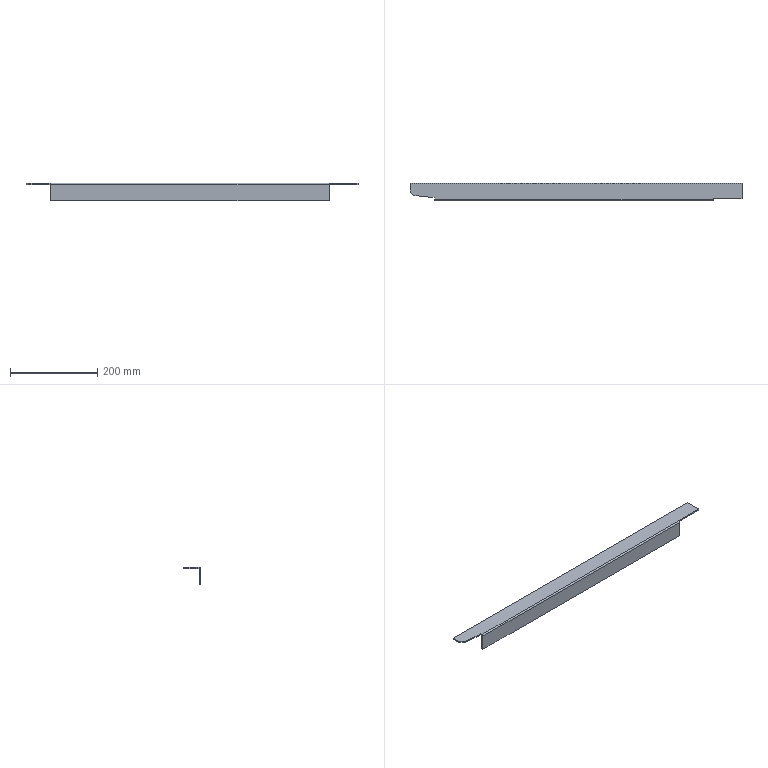Part | SolidWorks | 1 solid | 20 faces | box 759.5 x 40 x 40 mm | volume 157924 mm3 | plane 18 | cylinder 2 | commonest cylinder face diameters 0.2 x1 6.2 x1
STEP:
#1=CARTESIAN_POINT('',(313.75,4.,0.));
#2=VERTEX_POINT('',#1);
#3=CARTESIAN_POINT('',(313.75,3.1,0.));
#4=VERTEX_POINT('',#3);
#5=CARTESIAN_POINT('',(313.75,-6.,0.));
#6=DIRECTION('',(0.,-1.,0.));
#7=VECTOR('',#6,1000.);
#8=LINE('',#5,#7);
#9=EDGE_CURVE('',#2,#4,#8,.T.);
#10=ORIENTED_EDGE('',*,*,#9,.T.);
#11=CARTESIAN_POINT('',(313.75,3.1,-3.));
#12=VERTEX_POINT('',#11);
#13=CARTESIAN_POINT('',(313.75,3.1,0.));
#14=DIRECTION('',(0.,0.,-1.));
#15=VECTOR('',#14,1000.);
#16=LINE('',#13,#15);
#17=EDGE_CURVE('',#4,#12,#16,.T.);
#18=ORIENTED_EDGE('',*,*,#17,.T.);
#19=CARTESIAN_POINT('',(313.75,4.,-3.));
#20=VERTEX_POINT('',#19);
#21=CARTESIAN_POINT('',(313.75,40.,-3.));
#22=DIRECTION('',(0.,1.,0.));
#23=VECTOR('',#22,1000.);
#24=LINE('',#21,#23);
#25=EDGE_CURVE('',#12,#20,#24,.T.);
#26=ORIENTED_EDGE('',*,*,#25,.T.);
#27=CARTESIAN_POINT('',(313.75,4.,-40.));
#28=DIRECTION('',(0.,0.,1.));
#29=VECTOR('',#28,1000.);
#30=LINE('',#27,#29);
#31=EDGE_CURVE('',#20,#2,#30,.T.);
#32=ORIENTED_EDGE('',*,*,#31,.T.);
#33=EDGE_LOOP('',(#10,#18,#26,#32));
#34=FACE_OUTER_BOUND('',#33,.T.);
#35=CARTESIAN_POINT('',(313.75,-6.,-40.));
#36=DIRECTION('',(-1.,0.,0.));
#37=DIRECTION('',(0.,0.,1.));
#38=AXIS2_PLACEMENT_3D('',#35,#36,#37);
#39=PLANE('',#38);
#40=ADVANCED_FACE('',(#34),#39,.F.);
#41=CARTESIAN_POINT('',(313.75,3.,-40.));
#42=VERTEX_POINT('',#41);
#43=CARTESIAN_POINT('',(313.75,3.,-3.1));
#44=VERTEX_POINT('',#43);
#45=CARTESIAN_POINT('',(313.75,3.,0.));
#46=DIRECTION('',(0.,0.,1.));
#47=VECTOR('',#46,1000.);
#48=LINE('',#45,#47);
#49=EDGE_CURVE('',#42,#44,#48,.T.);
#50=ORIENTED_EDGE('',*,*,#49,.T.);
#51=CARTESIAN_POINT('',(313.75,0.,-3.1));
#52=VERTEX_POINT('',#51);
#53=CARTESIAN_POINT('',(313.75,3.,-3.1));
#54=DIRECTION('',(0.,-1.,0.));
#55=VECTOR('',#54,1000.);
#56=LINE('',#53,#55);
#57=EDGE_CURVE('',#44,#52,#56,.T.);
#58=ORIENTED_EDGE('',*,*,#57,.T.);
#59=CARTESIAN_POINT('',(313.75,0.,-40.));
#60=VERTEX_POINT('',#59);
#61=CARTESIAN_POINT('',(313.75,0.,0.));
#62=DIRECTION('',(0.,0.,1.));
#63=VECTOR('',#62,1000.);
#64=LINE('',#61,#63);
#65=EDGE_CURVE('',#60,#52,#64,.T.);
#66=ORIENTED_EDGE('',*,*,#65,.F.);
#67=CARTESIAN_POINT('',(313.75,-6.,-40.));
#68=DIRECTION('',(0.,-1.,0.));
#69=VECTOR('',#68,1000.);
#70=LINE('',#67,#69);
#71=EDGE_CURVE('',#42,#60,#70,.T.);
#72=ORIENTED_EDGE('',*,*,#71,.F.);
#73=EDGE_LOOP('',(#50,#58,#66,#72));
#74=FACE_OUTER_BOUND('',#73,.T.);
#75=CARTESIAN_POINT('',(313.75,-6.,-40.));
#76=DIRECTION('',(-1.,0.,0.));
#77=DIRECTION('',(0.,0.,1.));
#78=AXIS2_PLACEMENT_3D('',#75,#76,#77);
#79=PLANE('',#78);
#80=ADVANCED_FACE('',(#74),#79,.F.);
#81=CARTESIAN_POINT('',(-323.25,0.,-40.));
#82=VERTEX_POINT('',#81);
#83=CARTESIAN_POINT('',(379.75,0.,-40.));
#84=DIRECTION('',(-1.,0.,0.));
#85=VECTOR('',#84,1000.);
#86=LINE('',#83,#85);
#87=EDGE_CURVE('',#60,#82,#86,.T.);
#88=ORIENTED_EDGE('',*,*,#87,.F.);
#89=ORIENTED_EDGE('',*,*,#65,.T.);
#90=CARTESIAN_POINT('',(-323.25,0.,-3.1));
#91=VERTEX_POINT('',#90);
#92=CARTESIAN_POINT('',(379.75,0.,-3.1));
#93=DIRECTION('',(-1.,0.,0.));
#94=VECTOR('',#93,1000.);
#95=LINE('',#92,#94);
#96=EDGE_CURVE('',#52,#91,#95,.T.);
#97=ORIENTED_EDGE('',*,*,#96,.T.);
#98=CARTESIAN_POINT('',(-323.25,0.,0.));
#99=DIRECTION('',(0.,0.,-1.));
#100=VECTOR('',#99,1000.);
#101=LINE('',#98,#100);
#102=EDGE_CURVE('',#91,#82,#101,.T.);
#103=ORIENTED_EDGE('',*,*,#102,.T.);
#104=EDGE_LOOP('',(#88,#89,#97,#103));
#105=FACE_OUTER_BOUND('',#104,.T.);
#106=CARTESIAN_POINT('',(379.75,0.,0.));
#107=DIRECTION('',(0.,1.,0.));
#108=DIRECTION('',(0.,0.,1.));
#109=AXIS2_PLACEMENT_3D('',#106,#107,#108);
#110=PLANE('',#109);
#111=ADVANCED_FACE('',(#105),#110,.F.);
#112=ORIENTED_EDGE('',*,*,#71,.T.);
#113=ORIENTED_EDGE('',*,*,#87,.T.);
#114=CARTESIAN_POINT('',(-323.25,3.,-40.));
#115=VERTEX_POINT('',#114);
#116=CARTESIAN_POINT('',(-323.25,3.,-40.));
#117=DIRECTION('',(0.,-1.,0.));
#118=VECTOR('',#117,1000.);
#119=LINE('',#116,#118);
#120=EDGE_CURVE('',#115,#82,#119,.T.);
#121=ORIENTED_EDGE('',*,*,#120,.F.);
#122=CARTESIAN_POINT('',(379.75,3.,-40.));
#123=DIRECTION('',(-1.,0.,0.));
#124=VECTOR('',#123,1000.);
#125=LINE('',#122,#124);
#126=EDGE_CURVE('',#42,#115,#125,.T.);
#127=ORIENTED_EDGE('',*,*,#126,.F.);
#128=EDGE_LOOP('',(#112,#113,#121,#127));
#129=FACE_OUTER_BOUND('',#128,.T.);
#130=CARTESIAN_POINT('',(379.75,3.,-40.));
#131=DIRECTION('',(0.,0.,-1.));
#132=DIRECTION('',(-1.,0.,0.));
#133=AXIS2_PLACEMENT_3D('',#130,#131,#132);
#134=PLANE('',#133);
#135=ADVANCED_FACE('',(#129),#134,.T.);
#136=ORIENTED_EDGE('',*,*,#49,.F.);
#137=ORIENTED_EDGE('',*,*,#126,.T.);
#138=CARTESIAN_POINT('',(-323.25,3.,-3.1));
#139=VERTEX_POINT('',#138);
#140=CARTESIAN_POINT('',(-323.25,3.,0.));
#141=DIRECTION('',(0.,0.,-1.));
#142=VECTOR('',#141,1000.);
#143=LINE('',#140,#142);
#144=EDGE_CURVE('',#139,#115,#143,.T.);
#145=ORIENTED_EDGE('',*,*,#144,.F.);
#146=CARTESIAN_POINT('',(379.75,3.,-3.1));
#147=DIRECTION('',(-1.,0.,0.));
#148=VECTOR('',#147,1000.);
#149=LINE('',#146,#148);
#150=EDGE_CURVE('',#44,#139,#149,.T.);
#151=ORIENTED_EDGE('',*,*,#150,.F.);
#152=EDGE_LOOP('',(#136,#137,#145,#151));
#153=FACE_OUTER_BOUND('',#152,.T.);
#154=CARTESIAN_POINT('',(379.75,3.,0.));
#155=DIRECTION('',(0.,1.,0.));
#156=DIRECTION('',(0.,0.,1.));
#157=AXIS2_PLACEMENT_3D('',#154,#155,#156);
#158=PLANE('',#157);
#159=ADVANCED_FACE('',(#153),#158,.T.);
#160=CARTESIAN_POINT('',(313.75,3.1,-3.1));
#161=DIRECTION('',(-1.,0.,0.));
#162=DIRECTION('',(0.,0.,1.));
#163=AXIS2_PLACEMENT_3D('',#160,#161,#162);
#164=CIRCLE('',#163,0.1);
#165=EDGE_CURVE('',#44,#12,#164,.T.);
#166=ORIENTED_EDGE('',*,*,#165,.F.);
#167=ORIENTED_EDGE('',*,*,#150,.T.);
#168=CARTESIAN_POINT('',(-323.25,3.1,-3.));
#169=VERTEX_POINT('',#168);
#170=CARTESIAN_POINT('',(-323.25,3.1,-3.1));
#171=DIRECTION('',(1.,0.,0.));
#172=DIRECTION('',(0.,1.,0.));
#173=AXIS2_PLACEMENT_3D('',#170,#171,#172);
#174=CIRCLE('',#173,0.1);
#175=EDGE_CURVE('',#169,#139,#174,.T.);
#176=ORIENTED_EDGE('',*,*,#175,.F.);
#177=CARTESIAN_POINT('',(379.75,3.1,-3.));
#178=DIRECTION('',(-1.,0.,0.));
#179=VECTOR('',#178,1000.);
#180=LINE('',#177,#179);
#181=EDGE_CURVE('',#12,#169,#180,.T.);
#182=ORIENTED_EDGE('',*,*,#181,.F.);
#183=EDGE_LOOP('',(#166,#167,#176,#182));
#184=FACE_OUTER_BOUND('',#183,.T.);
#185=CARTESIAN_POINT('',(379.75,3.1,-3.1));
#186=DIRECTION('',(-1.,0.,0.));
#187=DIRECTION('',(0.,0.,1.));
#188=AXIS2_PLACEMENT_3D('',#185,#186,#187);
#189=CYLINDRICAL_SURFACE('',#188,0.1);
#190=ADVANCED_FACE('',(#184),#189,.F.);
#191=ORIENTED_EDGE('',*,*,#25,.F.);
#192=ORIENTED_EDGE('',*,*,#181,.T.);
#193=CARTESIAN_POINT('',(-323.25,7.501,-3.));
#194=VERTEX_POINT('',#193);
#195=CARTESIAN_POINT('',(-323.25,40.,-3.));
#196=DIRECTION('',(0.,-1.,0.));
#197=VECTOR('',#196,1000.);
#198=LINE('',#195,#197);
#199=EDGE_CURVE('',#194,#169,#198,.T.);
#200=ORIENTED_EDGE('',*,*,#199,.F.);
#201=CARTESIAN_POINT('',(-327.727,7.501,-3.));
#202=VERTEX_POINT('',#201);
#203=CARTESIAN_POINT('',(379.75,7.501,-3.));
#204=DIRECTION('',(1.,0.,0.));
#205=VECTOR('',#204,1000.);
#206=LINE('',#203,#205);
#207=EDGE_CURVE('',#202,#194,#206,.T.);
#208=ORIENTED_EDGE('',*,*,#207,.F.);
#209=CARTESIAN_POINT('',(-370.795,12.028,-3.));
#210=VERTEX_POINT('',#209);
#211=CARTESIAN_POINT('',(368.642,-65.69,-3.));
#212=DIRECTION('',(0.9945,-0.1045,0.));
#213=VECTOR('',#212,1000.);
#214=LINE('',#211,#213);
#215=EDGE_CURVE('',#210,#202,#214,.T.);
#216=ORIENTED_EDGE('',*,*,#215,.F.);
#217=CARTESIAN_POINT('',(-379.75,21.973,-3.));
#218=VERTEX_POINT('',#217);
#219=CARTESIAN_POINT('',(-48.659,-345.741,-3.));
#220=DIRECTION('',(0.6691,-0.7431,0.));
#221=VECTOR('',#220,1000.);
#222=LINE('',#219,#221);
#223=EDGE_CURVE('',#218,#210,#222,.T.);
#224=ORIENTED_EDGE('',*,*,#223,.F.);
#225=CARTESIAN_POINT('',(-379.75,40.,-3.));
#226=VERTEX_POINT('',#225);
#227=CARTESIAN_POINT('',(-379.75,40.,-3.));
#228=DIRECTION('',(0.,-1.,0.));
#229=VECTOR('',#228,1000.);
#230=LINE('',#227,#229);
#231=EDGE_CURVE('',#226,#218,#230,.T.);
#232=ORIENTED_EDGE('',*,*,#231,.F.);
#233=CARTESIAN_POINT('',(379.75,40.,-3.));
#234=VERTEX_POINT('',#233);
#235=CARTESIAN_POINT('',(379.75,40.,-3.));
#236=DIRECTION('',(-1.,0.,0.));
#237=VECTOR('',#236,1000.);
#238=LINE('',#235,#237);
#239=EDGE_CURVE('',#234,#226,#238,.T.);
#240=ORIENTED_EDGE('',*,*,#239,.F.);
#241=CARTESIAN_POINT('',(379.75,4.,-3.));
#242=VERTEX_POINT('',#241);
#243=CARTESIAN_POINT('',(379.75,40.,-3.));
#244=DIRECTION('',(0.,-1.,0.));
#245=VECTOR('',#244,1000.);
#246=LINE('',#243,#245);
#247=EDGE_CURVE('',#234,#242,#246,.T.);
#248=ORIENTED_EDGE('',*,*,#247,.T.);
#249=CARTESIAN_POINT('',(379.75,4.,-3.));
#250=DIRECTION('',(1.,0.,0.));
#251=VECTOR('',#250,1000.);
#252=LINE('',#249,#251);
#253=EDGE_CURVE('',#20,#242,#252,.T.);
#254=ORIENTED_EDGE('',*,*,#253,.F.);
#255=EDGE_LOOP('',(#191,#192,#200,#208,#216,#224,#232,#240,#248,#254));
#256=FACE_OUTER_BOUND('',#255,.T.);
#257=CARTESIAN_POINT('',(379.75,40.,-3.));
#258=DIRECTION('',(0.,0.,-1.));
#259=DIRECTION('',(0.,1.,0.));
#260=AXIS2_PLACEMENT_3D('',#257,#258,#259);
#261=PLANE('',#260);
#262=ADVANCED_FACE('',(#256),#261,.T.);
#263=CARTESIAN_POINT('',(-323.25,3.1,0.));
#264=VERTEX_POINT('',#263);
#265=CARTESIAN_POINT('',(379.75,3.1,0.));
#266=DIRECTION('',(-1.,0.,0.));
#267=VECTOR('',#266,1000.);
#268=LINE('',#265,#267);
#269=EDGE_CURVE('',#4,#264,#268,.T.);
#270=ORIENTED_EDGE('',*,*,#269,.F.);
#271=ORIENTED_EDGE('',*,*,#9,.F.);
#272=CARTESIAN_POINT('',(379.75,4.,0.));
#273=VERTEX_POINT('',#272);
#274=CARTESIAN_POINT('',(384.75,4.,0.));
#275=DIRECTION('',(-1.,0.,0.));
#276=VECTOR('',#275,1000.);
#277=LINE('',#274,#276);
#278=EDGE_CURVE('',#273,#2,#277,.T.);
#279=ORIENTED_EDGE('',*,*,#278,.F.);
#280=CARTESIAN_POINT('',(379.75,40.,0.));
#281=VERTEX_POINT('',#280);
#282=CARTESIAN_POINT('',(379.75,40.,0.));
#283=DIRECTION('',(0.,-1.,0.));
#284=VECTOR('',#283,1000.);
#285=LINE('',#282,#284);
#286=EDGE_CURVE('',#281,#273,#285,.T.);
#287=ORIENTED_EDGE('',*,*,#286,.F.);
#288=CARTESIAN_POINT('',(-379.75,40.,0.));
#289=VERTEX_POINT('',#288);
#290=CARTESIAN_POINT('',(379.75,40.,0.));
#291=DIRECTION('',(-1.,0.,0.));
#292=VECTOR('',#291,1000.);
#293=LINE('',#290,#292);
#294=EDGE_CURVE('',#281,#289,#293,.T.);
#295=ORIENTED_EDGE('',*,*,#294,.T.);
#296=CARTESIAN_POINT('',(-379.75,21.973,0.));
#297=VERTEX_POINT('',#296);
#298=CARTESIAN_POINT('',(-379.75,40.,0.));
#299=DIRECTION('',(0.,-1.,0.));
#300=VECTOR('',#299,1000.);
#301=LINE('',#298,#300);
#302=EDGE_CURVE('',#289,#297,#301,.T.);
#303=ORIENTED_EDGE('',*,*,#302,.T.);
#304=CARTESIAN_POINT('',(-370.795,12.028,0.));
#305=VERTEX_POINT('',#304);
#306=CARTESIAN_POINT('',(-48.659,-345.741,0.));
#307=DIRECTION('',(0.6691,-0.7431,0.));
#308=VECTOR('',#307,1000.);
#309=LINE('',#306,#308);
#310=EDGE_CURVE('',#297,#305,#309,.T.);
#311=ORIENTED_EDGE('',*,*,#310,.T.);
#312=CARTESIAN_POINT('',(-327.727,7.501,0.));
#313=VERTEX_POINT('',#312);
#314=CARTESIAN_POINT('',(368.642,-65.69,0.));
#315=DIRECTION('',(0.9945,-0.1045,0.));
#316=VECTOR('',#315,1000.);
#317=LINE('',#314,#316);
#318=EDGE_CURVE('',#305,#313,#317,.T.);
#319=ORIENTED_EDGE('',*,*,#318,.T.);
#320=CARTESIAN_POINT('',(-323.25,7.501,0.));
#321=VERTEX_POINT('',#320);
#322=CARTESIAN_POINT('',(379.75,7.501,0.));
#323=DIRECTION('',(1.,0.,0.));
#324=VECTOR('',#323,1000.);
#325=LINE('',#322,#324);
#326=EDGE_CURVE('',#313,#321,#325,.T.);
#327=ORIENTED_EDGE('',*,*,#326,.T.);
#328=CARTESIAN_POINT('',(-323.25,40.,0.));
#329=DIRECTION('',(0.,-1.,0.));
#330=VECTOR('',#329,1000.);
#331=LINE('',#328,#330);
#332=EDGE_CURVE('',#321,#264,#331,.T.);
#333=ORIENTED_EDGE('',*,*,#332,.T.);
#334=EDGE_LOOP('',(#270,#271,#279,#287,#295,#303,#311,#319,#327,#333));
#335=FACE_OUTER_BOUND('',#334,.T.);
#336=CARTESIAN_POINT('',(379.75,40.,0.));
#337=DIRECTION('',(0.,0.,-1.));
#338=DIRECTION('',(0.,1.,0.));
#339=AXIS2_PLACEMENT_3D('',#336,#337,#338);
#340=PLANE('',#339);
#341=ADVANCED_FACE('',(#335),#340,.F.);
#342=ORIENTED_EDGE('',*,*,#96,.F.);
#343=CARTESIAN_POINT('',(313.75,3.1,-3.1));
#344=DIRECTION('',(-1.,0.,0.));
#345=DIRECTION('',(0.,0.,1.));
#346=AXIS2_PLACEMENT_3D('',#343,#344,#345);
#347=CIRCLE('',#346,3.1);
#348=EDGE_CURVE('',#52,#4,#347,.T.);
#349=ORIENTED_EDGE('',*,*,#348,.T.);
#350=ORIENTED_EDGE('',*,*,#269,.T.);
#351=CARTESIAN_POINT('',(-323.25,3.1,-3.1));
#352=DIRECTION('',(1.,0.,0.));
#353=DIRECTION('',(0.,0.,1.));
#354=AXIS2_PLACEMENT_3D('',#351,#352,#353);
#355=CIRCLE('',#354,3.1);
#356=EDGE_CURVE('',#264,#91,#355,.T.);
#357=ORIENTED_EDGE('',*,*,#356,.T.);
#358=EDGE_LOOP('',(#342,#349,#350,#357));
#359=FACE_OUTER_BOUND('',#358,.T.);
#360=CARTESIAN_POINT('',(379.75,3.1,-3.1));
#361=DIRECTION('',(-1.,0.,0.));
#362=DIRECTION('',(0.,0.,1.));
#363=AXIS2_PLACEMENT_3D('',#360,#361,#362);
#364=CYLINDRICAL_SURFACE('',#363,3.1);
#365=ADVANCED_FACE('',(#359),#364,.T.);
#366=CARTESIAN_POINT('',(379.75,4.,-3.1));
#367=DIRECTION('',(0.,0.,1.));
#368=VECTOR('',#367,1000.);
#369=LINE('',#366,#368);
#370=EDGE_CURVE('',#242,#273,#369,.T.);
#371=ORIENTED_EDGE('',*,*,#370,.F.);
#372=ORIENTED_EDGE('',*,*,#247,.F.);
#373=CARTESIAN_POINT('',(379.75,40.,0.));
#374=DIRECTION('',(0.,0.,-1.));
#375=VECTOR('',#374,1000.);
#376=LINE('',#373,#375);
#377=EDGE_CURVE('',#281,#234,#376,.T.);
#378=ORIENTED_EDGE('',*,*,#377,.F.);
#379=ORIENTED_EDGE('',*,*,#286,.T.);
#380=EDGE_LOOP('',(#371,#372,#378,#379));
#381=FACE_OUTER_BOUND('',#380,.T.);
#382=CARTESIAN_POINT('',(379.75,3.,-3.1));
#383=DIRECTION('',(1.,0.,0.));
#384=DIRECTION('',(0.,0.,-1.));
#385=AXIS2_PLACEMENT_3D('',#382,#383,#384);
#386=PLANE('',#385);
#387=ADVANCED_FACE('',(#381),#386,.T.);
#388=CARTESIAN_POINT('',(-379.75,40.,0.));
#389=DIRECTION('',(0.,0.,-1.));
#390=VECTOR('',#389,1000.);
#391=LINE('',#388,#390);
#392=EDGE_CURVE('',#289,#226,#391,.T.);
#393=ORIENTED_EDGE('',*,*,#392,.F.);
#394=ORIENTED_EDGE('',*,*,#294,.F.);
#395=ORIENTED_EDGE('',*,*,#377,.T.);
#396=ORIENTED_EDGE('',*,*,#239,.T.);
#397=EDGE_LOOP('',(#393,#394,#395,#396));
#398=FACE_OUTER_BOUND('',#397,.T.);
#399=CARTESIAN_POINT('',(379.75,40.,0.));
#400=DIRECTION('',(0.,1.,0.));
#401=DIRECTION('',(0.,0.,1.));
#402=AXIS2_PLACEMENT_3D('',#399,#400,#401);
#403=PLANE('',#402);
#404=ADVANCED_FACE('',(#398),#403,.T.);
#405=CARTESIAN_POINT('',(-379.75,21.973,-3.));
#406=DIRECTION('',(0.,0.,1.));
#407=VECTOR('',#406,1000.);
#408=LINE('',#405,#407);
#409=EDGE_CURVE('',#218,#297,#408,.T.);
#410=ORIENTED_EDGE('',*,*,#409,.T.);
#411=ORIENTED_EDGE('',*,*,#302,.F.);
#412=ORIENTED_EDGE('',*,*,#392,.T.);
#413=ORIENTED_EDGE('',*,*,#231,.T.);
#414=EDGE_LOOP('',(#410,#411,#412,#413));
#415=FACE_OUTER_BOUND('',#414,.T.);
#416=CARTESIAN_POINT('',(-379.75,3.1,-3.1));
#417=DIRECTION('',(1.,0.,0.));
#418=DIRECTION('',(0.,0.,-1.));
#419=AXIS2_PLACEMENT_3D('',#416,#417,#418);
#420=PLANE('',#419);
#421=ADVANCED_FACE('',(#415),#420,.F.);
#422=ORIENTED_EDGE('',*,*,#144,.T.);
#423=ORIENTED_EDGE('',*,*,#120,.T.);
#424=ORIENTED_EDGE('',*,*,#102,.F.);
#425=CARTESIAN_POINT('',(-323.25,3.,-3.1));
#426=DIRECTION('',(0.,-1.,0.));
#427=VECTOR('',#426,1000.);
#428=LINE('',#425,#427);
#429=EDGE_CURVE('',#139,#91,#428,.T.);
#430=ORIENTED_EDGE('',*,*,#429,.F.);
#431=EDGE_LOOP('',(#422,#423,#424,#430));
#432=FACE_OUTER_BOUND('',#431,.T.);
#433=CARTESIAN_POINT('',(-323.25,3.,0.));
#434=DIRECTION('',(1.,0.,0.));
#435=DIRECTION('',(0.,0.,-1.));
#436=AXIS2_PLACEMENT_3D('',#433,#434,#435);
#437=PLANE('',#436);
#438=ADVANCED_FACE('',(#432),#437,.F.);
#439=ORIENTED_EDGE('',*,*,#409,.F.);
#440=ORIENTED_EDGE('',*,*,#223,.T.);
#441=CARTESIAN_POINT('',(-370.795,12.028,-3.));
#442=DIRECTION('',(0.,0.,1.));
#443=VECTOR('',#442,1000.);
#444=LINE('',#441,#443);
#445=EDGE_CURVE('',#210,#305,#444,.T.);
#446=ORIENTED_EDGE('',*,*,#445,.T.);
#447=ORIENTED_EDGE('',*,*,#310,.F.);
#448=EDGE_LOOP('',(#439,#440,#446,#447));
#449=FACE_OUTER_BOUND('',#448,.T.);
#450=CARTESIAN_POINT('',(-48.659,-345.741,-3.));
#451=DIRECTION('',(0.7431,0.6691,0.));
#452=DIRECTION('',(0.6691,-0.7431,0.));
#453=AXIS2_PLACEMENT_3D('',#450,#451,#452);
#454=PLANE('',#453);
#455=ADVANCED_FACE('',(#449),#454,.F.);
#456=ORIENTED_EDGE('',*,*,#445,.F.);
#457=ORIENTED_EDGE('',*,*,#215,.T.);
#458=CARTESIAN_POINT('',(-327.727,7.501,-3.));
#459=DIRECTION('',(0.,0.,1.));
#460=VECTOR('',#459,1000.);
#461=LINE('',#458,#460);
#462=EDGE_CURVE('',#202,#313,#461,.T.);
#463=ORIENTED_EDGE('',*,*,#462,.T.);
#464=ORIENTED_EDGE('',*,*,#318,.F.);
#465=EDGE_LOOP('',(#456,#457,#463,#464));
#466=FACE_OUTER_BOUND('',#465,.T.);
#467=CARTESIAN_POINT('',(368.642,-65.69,-3.));
#468=DIRECTION('',(0.1045,0.9945,0.));
#469=DIRECTION('',(0.9945,-0.1045,0.));
#470=AXIS2_PLACEMENT_3D('',#467,#468,#469);
#471=PLANE('',#470);
#472=ADVANCED_FACE('',(#466),#471,.F.);
#473=ORIENTED_EDGE('',*,*,#462,.F.);
#474=ORIENTED_EDGE('',*,*,#207,.T.);
#475=CARTESIAN_POINT('',(-323.25,7.501,-3.));
#476=DIRECTION('',(0.,0.,1.));
#477=VECTOR('',#476,1000.);
#478=LINE('',#475,#477);
#479=EDGE_CURVE('',#194,#321,#478,.T.);
#480=ORIENTED_EDGE('',*,*,#479,.T.);
#481=ORIENTED_EDGE('',*,*,#326,.F.);
#482=EDGE_LOOP('',(#473,#474,#480,#481));
#483=FACE_OUTER_BOUND('',#482,.T.);
#484=CARTESIAN_POINT('',(379.75,7.501,-3.));
#485=DIRECTION('',(0.,1.,0.));
#486=DIRECTION('',(1.,0.,0.));
#487=AXIS2_PLACEMENT_3D('',#484,#485,#486);
#488=PLANE('',#487);
#489=ADVANCED_FACE('',(#483),#488,.F.);
#490=ORIENTED_EDGE('',*,*,#199,.T.);
#491=CARTESIAN_POINT('',(-323.25,3.1,-3.));
#492=DIRECTION('',(0.,0.,1.));
#493=VECTOR('',#492,1000.);
#494=LINE('',#491,#493);
#495=EDGE_CURVE('',#169,#264,#494,.T.);
#496=ORIENTED_EDGE('',*,*,#495,.T.);
#497=ORIENTED_EDGE('',*,*,#332,.F.);
#498=ORIENTED_EDGE('',*,*,#479,.F.);
#499=EDGE_LOOP('',(#490,#496,#497,#498));
#500=FACE_OUTER_BOUND('',#499,.T.);
#501=CARTESIAN_POINT('',(-323.25,40.,-3.));
#502=DIRECTION('',(1.,0.,0.));
#503=DIRECTION('',(0.,-1.,0.));
#504=AXIS2_PLACEMENT_3D('',#501,#502,#503);
#505=PLANE('',#504);
#506=ADVANCED_FACE('',(#500),#505,.F.);
#507=ORIENTED_EDGE('',*,*,#175,.T.);
#508=ORIENTED_EDGE('',*,*,#429,.T.);
#509=ORIENTED_EDGE('',*,*,#356,.F.);
#510=ORIENTED_EDGE('',*,*,#495,.F.);
#511=EDGE_LOOP('',(#507,#508,#509,#510));
#512=FACE_OUTER_BOUND('',#511,.T.);
#513=CARTESIAN_POINT('',(-323.25,3.1,-3.1));
#514=DIRECTION('',(-1.,0.,0.));
#515=DIRECTION('',(0.,-1.,0.));
#516=AXIS2_PLACEMENT_3D('',#513,#514,#515);
#517=PLANE('',#516);
#518=ADVANCED_FACE('',(#512),#517,.T.);
#519=ORIENTED_EDGE('',*,*,#17,.F.);
#520=ORIENTED_EDGE('',*,*,#348,.F.);
#521=ORIENTED_EDGE('',*,*,#57,.F.);
#522=ORIENTED_EDGE('',*,*,#165,.T.);
#523=EDGE_LOOP('',(#519,#520,#521,#522));
#524=FACE_OUTER_BOUND('',#523,.T.);
#525=CARTESIAN_POINT('',(313.75,-6.,-40.));
#526=DIRECTION('',(-1.,0.,0.));
#527=DIRECTION('',(0.,0.,1.));
#528=AXIS2_PLACEMENT_3D('',#525,#526,#527);
#529=PLANE('',#528);
#530=ADVANCED_FACE('',(#524),#529,.F.);
#531=ORIENTED_EDGE('',*,*,#253,.T.);
#532=ORIENTED_EDGE('',*,*,#370,.T.);
#533=ORIENTED_EDGE('',*,*,#278,.T.);
#534=ORIENTED_EDGE('',*,*,#31,.F.);
#535=EDGE_LOOP('',(#531,#532,#533,#534));
#536=FACE_OUTER_BOUND('',#535,.T.);
#537=CARTESIAN_POINT('',(384.75,4.,-40.));
#538=DIRECTION('',(0.,1.,0.));
#539=DIRECTION('',(-1.,0.,0.));
#540=AXIS2_PLACEMENT_3D('',#537,#538,#539);
#541=PLANE('',#540);
#542=ADVANCED_FACE('',(#536),#541,.F.);
#543=CLOSED_SHELL('',(#40,#80,#111,#135,#159,#190,#262,#341,#365,#387,#404,#421,#438,#455,#472,#489,#506,#518,#530,#542));
#544=MANIFOLD_SOLID_BREP('',#543);
#545=CARTESIAN_POINT('',(0.,0.,0.));
#546=DIRECTION('',(0.,0.,1.));
#547=DIRECTION('',(1.,0.,0.));
#548=AXIS2_PLACEMENT_3D('',#545,#546,#547);
#549=(LENGTH_UNIT()NAMED_UNIT(*)SI_UNIT(.MILLI.,.METRE.));
#550=UNCERTAINTY_MEASURE_WITH_UNIT(LENGTH_MEASURE(0.00001),#549,'','');
#551=(NAMED_UNIT(*)PLANE_ANGLE_UNIT()SI_UNIT($,.RADIAN.));
#552=(NAMED_UNIT(*)SI_UNIT($,.STERADIAN.)SOLID_ANGLE_UNIT());
#553=(GEOMETRIC_REPRESENTATION_CONTEXT(3)GLOBAL_UNCERTAINTY_ASSIGNED_CONTEXT((#550))GLOBAL_UNIT_ASSIGNED_CONTEXT((#549,#551,#552))REPRESENTATION_CONTEXT('',''));
#554=ADVANCED_BREP_SHAPE_REPRESENTATION('',(#544,#548),#553);